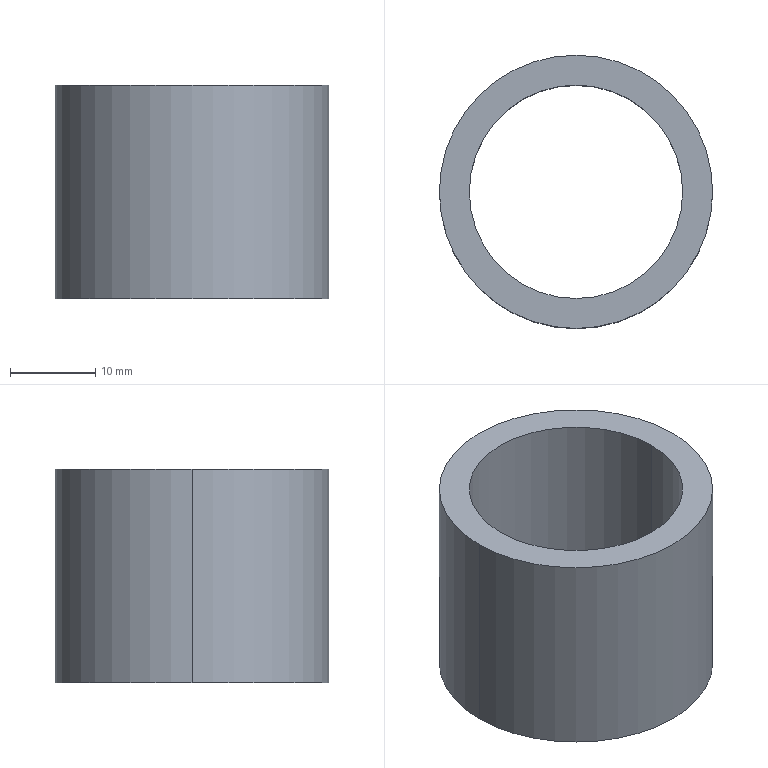Part | SolidWorks | features BaseBody 1 | 1 solid | 6 faces | box 32 x 32 x 25 mm | volume 7834 mm3 | cylinder 4 | plane 2 | commonest cylinder face diameters 25 x2 32 x2
STEP:
#1=CARTESIAN_POINT('',(162.047,1592.079,-1156.));
#2=VERTEX_POINT('',#1);
#3=CARTESIAN_POINT('',(194.047,1592.079,-1156.));
#4=VERTEX_POINT('',#3);
#5=CARTESIAN_POINT('',(178.047,1592.079,-1156.));
#6=DIRECTION('',(0.,0.,-1.));
#7=DIRECTION('',(-1.,0.,0.));
#8=AXIS2_PLACEMENT_3D('',#5,#6,#7);
#9=CIRCLE('',#8,16.);
#10=EDGE_CURVE('',#2,#4,#9,.T.);
#11=ORIENTED_EDGE('',*,*,#10,.T.);
#12=CARTESIAN_POINT('',(194.047,1592.079,-1181.));
#13=VERTEX_POINT('',#12);
#14=CARTESIAN_POINT('',(194.047,1592.079,-1171.));
#15=DIRECTION('',(0.,0.,-1.));
#16=VECTOR('',#15,1000.);
#17=LINE('',#14,#16);
#18=EDGE_CURVE('',#4,#13,#17,.T.);
#19=ORIENTED_EDGE('',*,*,#18,.T.);
#20=CARTESIAN_POINT('',(162.047,1592.079,-1181.));
#21=VERTEX_POINT('',#20);
#22=CARTESIAN_POINT('',(178.047,1592.079,-1181.));
#23=DIRECTION('',(0.,0.,1.));
#24=DIRECTION('',(-1.,0.,0.));
#25=AXIS2_PLACEMENT_3D('',#22,#23,#24);
#26=CIRCLE('',#25,16.);
#27=EDGE_CURVE('',#13,#21,#26,.T.);
#28=ORIENTED_EDGE('',*,*,#27,.T.);
#29=CARTESIAN_POINT('',(162.047,1592.079,-1171.));
#30=DIRECTION('',(0.,0.,-1.));
#31=VECTOR('',#30,1000.);
#32=LINE('',#29,#31);
#33=EDGE_CURVE('',#2,#21,#32,.T.);
#34=ORIENTED_EDGE('',*,*,#33,.F.);
#35=EDGE_LOOP('',(#11,#19,#28,#34));
#36=FACE_OUTER_BOUND('',#35,.T.);
#37=CARTESIAN_POINT('',(178.047,1592.079,-1171.));
#38=DIRECTION('',(0.,0.,-1.));
#39=DIRECTION('',(-1.,0.,0.));
#40=AXIS2_PLACEMENT_3D('',#37,#38,#39);
#41=CYLINDRICAL_SURFACE('',#40,16.);
#42=ADVANCED_FACE('',(#36),#41,.T.);
#43=CARTESIAN_POINT('',(165.547,1592.079,-1156.));
#44=VERTEX_POINT('',#43);
#45=CARTESIAN_POINT('',(190.547,1592.079,-1156.));
#46=VERTEX_POINT('',#45);
#47=CARTESIAN_POINT('',(178.047,1592.079,-1156.));
#48=DIRECTION('',(0.,0.,1.));
#49=DIRECTION('',(-1.,0.,0.));
#50=AXIS2_PLACEMENT_3D('',#47,#48,#49);
#51=CIRCLE('',#50,12.5);
#52=EDGE_CURVE('',#44,#46,#51,.T.);
#53=ORIENTED_EDGE('',*,*,#52,.T.);
#54=CARTESIAN_POINT('',(190.547,1592.079,-1181.));
#55=VERTEX_POINT('',#54);
#56=CARTESIAN_POINT('',(190.547,1592.079,-1171.));
#57=DIRECTION('',(0.,0.,-1.));
#58=VECTOR('',#57,1000.);
#59=LINE('',#56,#58);
#60=EDGE_CURVE('',#46,#55,#59,.T.);
#61=ORIENTED_EDGE('',*,*,#60,.T.);
#62=CARTESIAN_POINT('',(165.547,1592.079,-1181.));
#63=VERTEX_POINT('',#62);
#64=CARTESIAN_POINT('',(178.047,1592.079,-1181.));
#65=DIRECTION('',(0.,0.,-1.));
#66=DIRECTION('',(-1.,0.,0.));
#67=AXIS2_PLACEMENT_3D('',#64,#65,#66);
#68=CIRCLE('',#67,12.5);
#69=EDGE_CURVE('',#55,#63,#68,.T.);
#70=ORIENTED_EDGE('',*,*,#69,.T.);
#71=CARTESIAN_POINT('',(165.547,1592.079,-1171.));
#72=DIRECTION('',(0.,0.,-1.));
#73=VECTOR('',#72,1000.);
#74=LINE('',#71,#73);
#75=EDGE_CURVE('',#44,#63,#74,.T.);
#76=ORIENTED_EDGE('',*,*,#75,.F.);
#77=EDGE_LOOP('',(#53,#61,#70,#76));
#78=FACE_OUTER_BOUND('',#77,.T.);
#79=CARTESIAN_POINT('',(178.047,1592.079,-1171.));
#80=DIRECTION('',(0.,0.,-1.));
#81=DIRECTION('',(-1.,0.,0.));
#82=AXIS2_PLACEMENT_3D('',#79,#80,#81);
#83=CYLINDRICAL_SURFACE('',#82,12.5);
#84=ADVANCED_FACE('',(#78),#83,.F.);
#85=ORIENTED_EDGE('',*,*,#18,.F.);
#86=CARTESIAN_POINT('',(178.047,1592.079,-1156.));
#87=DIRECTION('',(0.,0.,-1.));
#88=DIRECTION('',(-1.,0.,0.));
#89=AXIS2_PLACEMENT_3D('',#86,#87,#88);
#90=CIRCLE('',#89,16.);
#91=EDGE_CURVE('',#4,#2,#90,.T.);
#92=ORIENTED_EDGE('',*,*,#91,.T.);
#93=ORIENTED_EDGE('',*,*,#33,.T.);
#94=CARTESIAN_POINT('',(178.047,1592.079,-1181.));
#95=DIRECTION('',(0.,0.,1.));
#96=DIRECTION('',(-1.,0.,0.));
#97=AXIS2_PLACEMENT_3D('',#94,#95,#96);
#98=CIRCLE('',#97,16.);
#99=EDGE_CURVE('',#21,#13,#98,.T.);
#100=ORIENTED_EDGE('',*,*,#99,.T.);
#101=EDGE_LOOP('',(#85,#92,#93,#100));
#102=FACE_OUTER_BOUND('',#101,.T.);
#103=CARTESIAN_POINT('',(178.047,1592.079,-1171.));
#104=DIRECTION('',(0.,0.,-1.));
#105=DIRECTION('',(-1.,0.,0.));
#106=AXIS2_PLACEMENT_3D('',#103,#104,#105);
#107=CYLINDRICAL_SURFACE('',#106,16.);
#108=ADVANCED_FACE('',(#102),#107,.T.);
#109=CARTESIAN_POINT('',(178.047,1592.079,-1181.));
#110=DIRECTION('',(0.,0.,-1.));
#111=DIRECTION('',(-1.,0.,0.));
#112=AXIS2_PLACEMENT_3D('',#109,#110,#111);
#113=CIRCLE('',#112,12.5);
#114=EDGE_CURVE('',#63,#55,#113,.T.);
#115=ORIENTED_EDGE('',*,*,#114,.F.);
#116=ORIENTED_EDGE('',*,*,#69,.F.);
#117=EDGE_LOOP('',(#115,#116));
#118=FACE_BOUND('',#117,.T.);
#119=ORIENTED_EDGE('',*,*,#99,.F.);
#120=ORIENTED_EDGE('',*,*,#27,.F.);
#121=EDGE_LOOP('',(#119,#120));
#122=FACE_OUTER_BOUND('',#121,.T.);
#123=CARTESIAN_POINT('',(193.604,1595.817,-1181.));
#124=DIRECTION('',(0.,0.,1.));
#125=DIRECTION('',(1.,0.,0.));
#126=AXIS2_PLACEMENT_3D('',#123,#124,#125);
#127=PLANE('',#126);
#128=ADVANCED_FACE('',(#118,#122),#127,.F.);
#129=ORIENTED_EDGE('',*,*,#52,.F.);
#130=CARTESIAN_POINT('',(178.047,1592.079,-1156.));
#131=DIRECTION('',(0.,0.,1.));
#132=DIRECTION('',(-1.,0.,0.));
#133=AXIS2_PLACEMENT_3D('',#130,#131,#132);
#134=CIRCLE('',#133,12.5);
#135=EDGE_CURVE('',#46,#44,#134,.T.);
#136=ORIENTED_EDGE('',*,*,#135,.F.);
#137=EDGE_LOOP('',(#129,#136));
#138=FACE_BOUND('',#137,.T.);
#139=ORIENTED_EDGE('',*,*,#10,.F.);
#140=ORIENTED_EDGE('',*,*,#91,.F.);
#141=EDGE_LOOP('',(#139,#140));
#142=FACE_OUTER_BOUND('',#141,.T.);
#143=CARTESIAN_POINT('',(190.201,1594.999,-1156.));
#144=DIRECTION('',(0.,0.,-1.));
#145=DIRECTION('',(-1.,0.,0.));
#146=AXIS2_PLACEMENT_3D('',#143,#144,#145);
#147=PLANE('',#146);
#148=ADVANCED_FACE('',(#138,#142),#147,.F.);
#149=ORIENTED_EDGE('',*,*,#60,.F.);
#150=ORIENTED_EDGE('',*,*,#135,.T.);
#151=ORIENTED_EDGE('',*,*,#75,.T.);
#152=ORIENTED_EDGE('',*,*,#114,.T.);
#153=EDGE_LOOP('',(#149,#150,#151,#152));
#154=FACE_OUTER_BOUND('',#153,.T.);
#155=CARTESIAN_POINT('',(178.047,1592.079,-1171.));
#156=DIRECTION('',(0.,0.,-1.));
#157=DIRECTION('',(-1.,0.,0.));
#158=AXIS2_PLACEMENT_3D('',#155,#156,#157);
#159=CYLINDRICAL_SURFACE('',#158,12.5);
#160=ADVANCED_FACE('',(#154),#159,.F.);
#161=CLOSED_SHELL('',(#42,#84,#108,#128,#148,#160));
#162=MANIFOLD_SOLID_BREP('',#161);
#163=CARTESIAN_POINT('',(0.,0.,0.));
#164=DIRECTION('',(0.,0.,1.));
#165=DIRECTION('',(1.,0.,0.));
#166=AXIS2_PLACEMENT_3D('',#163,#164,#165);
#167=(LENGTH_UNIT()NAMED_UNIT(*)SI_UNIT(.MILLI.,.METRE.));
#168=UNCERTAINTY_MEASURE_WITH_UNIT(LENGTH_MEASURE(0.00001),#167,'','');
#169=(NAMED_UNIT(*)PLANE_ANGLE_UNIT()SI_UNIT($,.RADIAN.));
#170=(NAMED_UNIT(*)SI_UNIT($,.STERADIAN.)SOLID_ANGLE_UNIT());
#171=(GEOMETRIC_REPRESENTATION_CONTEXT(3)GLOBAL_UNCERTAINTY_ASSIGNED_CONTEXT((#168))GLOBAL_UNIT_ASSIGNED_CONTEXT((#167,#169,#170))REPRESENTATION_CONTEXT('',''));
#172=ADVANCED_BREP_SHAPE_REPRESENTATION('',(#162,#166),#171);